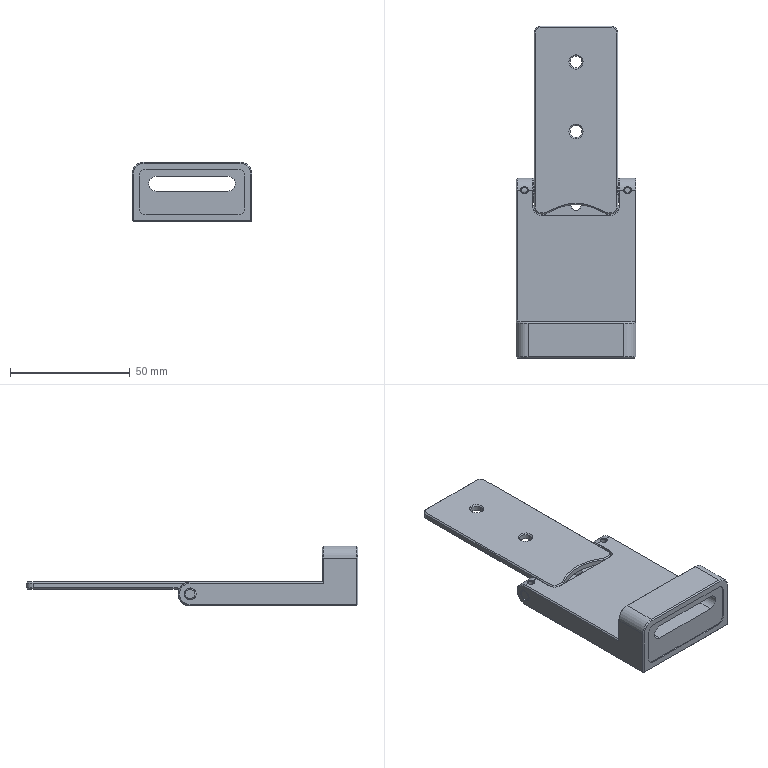Part | SolidWorks | 5 solids | 209 faces | box 50 x 138.5 x 25 mm | volume 43110 mm3 | plane 73 | cone 72 | cylinder 64 | commonest cylinder face diameters 5 x14 6 x14 10 x10 4 x7 2.5 x6 7 x4